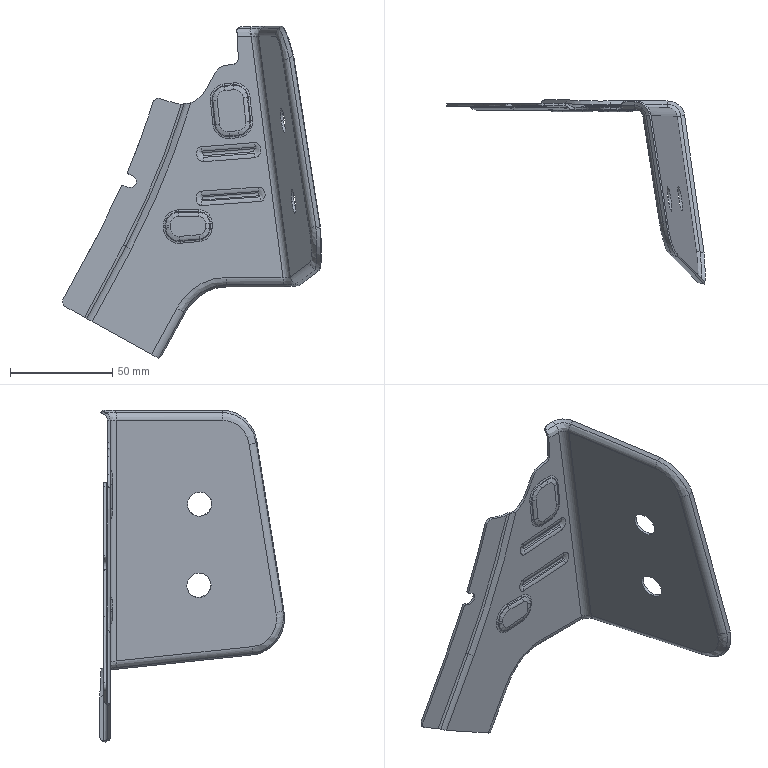Part | STEP file | FNA5401131 | 1 solid | 268 faces | box 126.55 x 90.381 x 162.439 mm | volume 23457 mm3 | spline 185 | cylinder 49 | plane 26 | other 8 | commonest cylinder face diameters 6 x17 3.6 x8 8.4 x7 8 x4 10.4 x4 12 x4